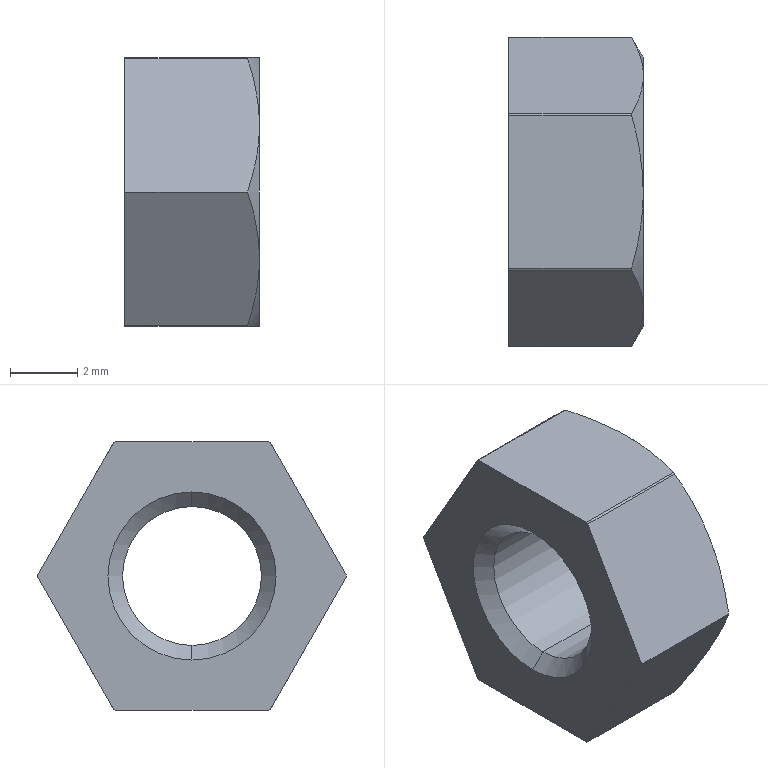Part | STEP file | Sceond2_8 | 1 solid | 24 faces | box 4 x 9.2 x 8 mm | volume 164.255 mm3 | cone 10 | plane 8 | cylinder 6 | commonest cylinder face diameters 9.2 x4 4.134 x2